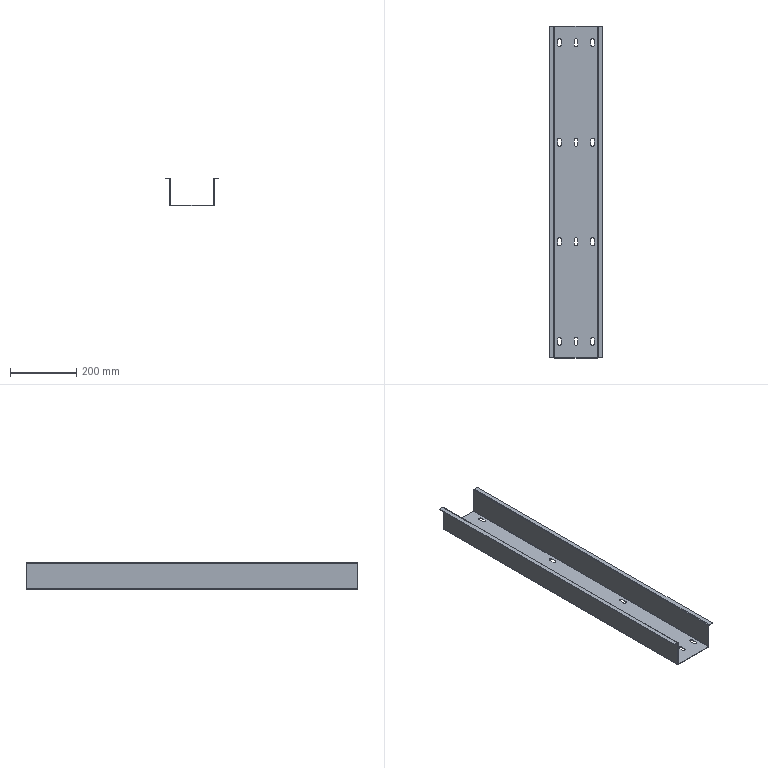Part | SolidWorks | features BaseBody 1 | 1 solid | 86 faces | box 160 x 1000 x 81.5 mm | volume 472667 mm3 | plane 54 | cylinder 32 | commonest cylinder face diameters 10 x24 1 x4 4 x4